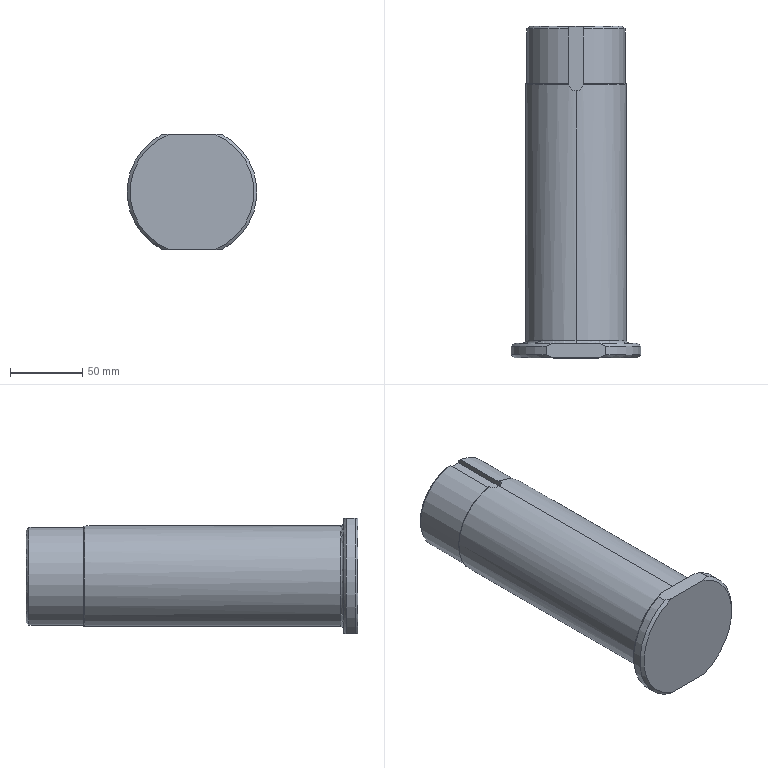Part | SolidWorks | features Fillet 3, ICE 2, Chamfer 1, Revolution 1 | 1 solid | 27 faces | box 90 x 230 x 80 mm | volume 896064 mm3 | plane 9 | cylinder 8 | cone 6 | torus 4 | commonest cylinder face diameters 10 x2 68 x2 70 x2 90 x2
STEP:
#1=CARTESIAN_POINT('',(0.,190.,-34.5));
#2=VERTEX_POINT('',#1);
#3=CARTESIAN_POINT('',(-5.,190.,34.136));
#4=VERTEX_POINT('',#3);
#5=CARTESIAN_POINT('',(0.,190.,0.));
#6=DIRECTION('',(0.,1.,0.));
#7=DIRECTION('',(0.,0.,-1.));
#8=AXIS2_PLACEMENT_3D('',#5,#6,#7);
#9=CIRCLE('',#8,34.5);
#10=EDGE_CURVE('',#2,#4,#9,.T.);
#11=ORIENTED_EDGE('',*,*,#10,.F.);
#12=CARTESIAN_POINT('',(0.,189.5,-35.));
#13=VERTEX_POINT('',#12);
#14=CARTESIAN_POINT('',(0.,189.5,-34.5));
#15=DIRECTION('',(-1.,0.,0.));
#16=DIRECTION('',(0.,0.,1.));
#17=AXIS2_PLACEMENT_3D('',#14,#15,#16);
#18=CIRCLE('',#17,0.5);
#19=EDGE_CURVE('',#2,#13,#18,.T.);
#20=ORIENTED_EDGE('',*,*,#19,.T.);
#21=CARTESIAN_POINT('',(-4.975,189.5,34.645));
#22=VERTEX_POINT('',#21);
#23=CARTESIAN_POINT('',(0.,189.5,0.));
#24=DIRECTION('',(0.,-1.,0.));
#25=DIRECTION('',(0.,0.,-1.));
#26=AXIS2_PLACEMENT_3D('',#23,#24,#25);
#27=CIRCLE('',#26,35.);
#28=EDGE_CURVE('',#22,#13,#27,.T.);
#29=ORIENTED_EDGE('',*,*,#28,.F.);
#30=CARTESIAN_POINT('',(-4.975,189.5,34.645));
#31=CARTESIAN_POINT('',(-4.988,189.632,34.643));
#32=CARTESIAN_POINT('',(-4.995,189.762,34.587));
#33=CARTESIAN_POINT('',(-5.001,189.946,34.399));
#34=CARTESIAN_POINT('',(-5.,190.,34.269));
#35=CARTESIAN_POINT('',(-5.,190.,34.136));
#36=B_SPLINE_CURVE_WITH_KNOTS('',3,(#30,#31,#32,#33,#34,#35),.UNSPECIFIED.,.F.,.F.,(4,2,4),(0.,0.0003936,0.0007872),.UNSPECIFIED.);
#37=EDGE_CURVE('',#22,#4,#36,.T.);
#38=ORIENTED_EDGE('',*,*,#37,.T.);
#39=EDGE_LOOP('',(#11,#20,#29,#38));
#40=FACE_OUTER_BOUND('',#39,.T.);
#41=CARTESIAN_POINT('',(0.,189.5,0.));
#42=DIRECTION('',(0.,-1.,0.));
#43=DIRECTION('',(0.,0.,-1.));
#44=AXIS2_PLACEMENT_3D('',#41,#42,#43);
#45=TOROIDAL_SURFACE('',#44,34.5,0.5);
#46=ADVANCED_FACE('',(#40),#45,.T.);
#47=CARTESIAN_POINT('',(0.,10.,37.));
#48=VERTEX_POINT('',#47);
#49=CARTESIAN_POINT('',(0.,10.,-37.));
#50=VERTEX_POINT('',#49);
#51=CARTESIAN_POINT('',(0.,10.,0.));
#52=DIRECTION('',(0.,-1.,0.));
#53=DIRECTION('',(0.,0.,-1.));
#54=AXIS2_PLACEMENT_3D('',#51,#52,#53);
#55=CIRCLE('',#54,37.);
#56=EDGE_CURVE('',#48,#50,#55,.T.);
#57=ORIENTED_EDGE('',*,*,#56,.F.);
#58=CARTESIAN_POINT('',(0.,12.,35.));
#59=VERTEX_POINT('',#58);
#60=CARTESIAN_POINT('',(0.,12.,37.));
#61=DIRECTION('',(1.,0.,0.));
#62=DIRECTION('',(0.,0.,-1.));
#63=AXIS2_PLACEMENT_3D('',#60,#61,#62);
#64=CIRCLE('',#63,2.);
#65=EDGE_CURVE('',#48,#59,#64,.T.);
#66=ORIENTED_EDGE('',*,*,#65,.T.);
#67=CARTESIAN_POINT('',(0.,12.,-35.));
#68=VERTEX_POINT('',#67);
#69=CARTESIAN_POINT('',(0.,12.,0.));
#70=DIRECTION('',(0.,1.,0.));
#71=DIRECTION('',(0.,0.,-1.));
#72=AXIS2_PLACEMENT_3D('',#69,#70,#71);
#73=CIRCLE('',#72,35.);
#74=EDGE_CURVE('',#68,#59,#73,.T.);
#75=ORIENTED_EDGE('',*,*,#74,.F.);
#76=CARTESIAN_POINT('',(0.,12.,-37.));
#77=DIRECTION('',(-1.,0.,0.));
#78=DIRECTION('',(0.,0.,1.));
#79=AXIS2_PLACEMENT_3D('',#76,#77,#78);
#80=CIRCLE('',#79,2.);
#81=EDGE_CURVE('',#50,#68,#80,.T.);
#82=ORIENTED_EDGE('',*,*,#81,.F.);
#83=EDGE_LOOP('',(#57,#66,#75,#82));
#84=FACE_OUTER_BOUND('',#83,.T.);
#85=CARTESIAN_POINT('',(0.,12.,0.));
#86=DIRECTION('',(0.,-1.,0.));
#87=DIRECTION('',(0.,0.,-1.));
#88=AXIS2_PLACEMENT_3D('',#85,#86,#87);
#89=TOROIDAL_SURFACE('',#88,37.,2.);
#90=ADVANCED_FACE('',(#84),#89,.F.);
#91=CARTESIAN_POINT('',(0.,230.,-32.));
#92=VERTEX_POINT('',#91);
#93=CARTESIAN_POINT('',(-5.,230.,31.607));
#94=VERTEX_POINT('',#93);
#95=CARTESIAN_POINT('',(0.,230.,0.));
#96=DIRECTION('',(0.,1.,0.));
#97=DIRECTION('',(0.,0.,-1.));
#98=AXIS2_PLACEMENT_3D('',#95,#96,#97);
#99=CIRCLE('',#98,32.);
#100=EDGE_CURVE('',#92,#94,#99,.T.);
#101=ORIENTED_EDGE('',*,*,#100,.F.);
#102=CARTESIAN_POINT('',(0.,228.,-34.));
#103=VERTEX_POINT('',#102);
#104=CARTESIAN_POINT('',(0.,228.,-34.));
#105=DIRECTION('',(0.,-0.7071,-0.7071));
#106=VECTOR('',#105,1000.);
#107=LINE('',#104,#106);
#108=EDGE_CURVE('',#92,#103,#107,.T.);
#109=ORIENTED_EDGE('',*,*,#108,.T.);
#110=CARTESIAN_POINT('',(-5.,228.,33.63));
#111=VERTEX_POINT('',#110);
#112=CARTESIAN_POINT('',(0.,228.,0.));
#113=DIRECTION('',(0.,-1.,0.));
#114=DIRECTION('',(0.,0.,-1.));
#115=AXIS2_PLACEMENT_3D('',#112,#113,#114);
#116=CIRCLE('',#115,34.);
#117=EDGE_CURVE('',#111,#103,#116,.T.);
#118=ORIENTED_EDGE('',*,*,#117,.F.);
#119=CARTESIAN_POINT('',(-5.,230.,31.607));
#120=CARTESIAN_POINT('',(-5.,229.334,32.282));
#121=CARTESIAN_POINT('',(-5.,228.667,32.956));
#122=CARTESIAN_POINT('',(-5.,228.,33.63));
#123=B_SPLINE_CURVE_WITH_KNOTS('',3,(#119,#120,#121,#122),.UNSPECIFIED.,.F.,.F.,(4,4),(0.006371,0.009216),.UNSPECIFIED.);
#124=EDGE_CURVE('',#94,#111,#123,.T.);
#125=ORIENTED_EDGE('',*,*,#124,.F.);
#126=EDGE_LOOP('',(#101,#109,#118,#125));
#127=FACE_OUTER_BOUND('',#126,.T.);
#128=CARTESIAN_POINT('',(0.,228.,0.));
#129=DIRECTION('',(0.,-1.,0.));
#130=DIRECTION('',(0.,0.,-1.));
#131=AXIS2_PLACEMENT_3D('',#128,#129,#130);
#132=CONICAL_SURFACE('',#131,34.,0.7854);
#133=ADVANCED_FACE('',(#127),#132,.T.);
#134=ORIENTED_EDGE('',*,*,#117,.T.);
#135=CARTESIAN_POINT('',(0.,190.,-34.));
#136=VERTEX_POINT('',#135);
#137=CARTESIAN_POINT('',(0.,0.,-34.));
#138=DIRECTION('',(0.,-1.,0.));
#139=VECTOR('',#138,1000.);
#140=LINE('',#137,#139);
#141=EDGE_CURVE('',#103,#136,#140,.T.);
#142=ORIENTED_EDGE('',*,*,#141,.T.);
#143=CARTESIAN_POINT('',(-5.,190.,33.63));
#144=VERTEX_POINT('',#143);
#145=CARTESIAN_POINT('',(0.,190.,0.));
#146=DIRECTION('',(0.,-1.,0.));
#147=DIRECTION('',(0.,0.,-1.));
#148=AXIS2_PLACEMENT_3D('',#145,#146,#147);
#149=CIRCLE('',#148,34.);
#150=EDGE_CURVE('',#144,#136,#149,.T.);
#151=ORIENTED_EDGE('',*,*,#150,.F.);
#152=CARTESIAN_POINT('',(-5.,0.,33.63));
#153=DIRECTION('',(0.,-1.,0.));
#154=VECTOR('',#153,1000.);
#155=LINE('',#152,#154);
#156=EDGE_CURVE('',#111,#144,#155,.T.);
#157=ORIENTED_EDGE('',*,*,#156,.F.);
#158=EDGE_LOOP('',(#134,#142,#151,#157));
#159=FACE_OUTER_BOUND('',#158,.T.);
#160=CARTESIAN_POINT('',(0.,0.,0.));
#161=DIRECTION('',(0.,-1.,0.));
#162=DIRECTION('',(0.,0.,-1.));
#163=AXIS2_PLACEMENT_3D('',#160,#161,#162);
#164=CYLINDRICAL_SURFACE('',#163,34.);
#165=ADVANCED_FACE('',(#159),#164,.T.);
#166=CARTESIAN_POINT('',(4.975,189.5,34.645));
#167=VERTEX_POINT('',#166);
#168=CARTESIAN_POINT('',(0.,185.,35.));
#169=VERTEX_POINT('',#168);
#170=CARTESIAN_POINT('',(4.975,189.5,34.645));
#171=CARTESIAN_POINT('',(4.944,189.192,34.649));
#172=CARTESIAN_POINT('',(4.885,188.892,34.658));
#173=CARTESIAN_POINT('',(4.714,188.306,34.681));
#174=CARTESIAN_POINT('',(4.601,188.019,34.697));
#175=CARTESIAN_POINT('',(4.324,187.47,34.732));
#176=CARTESIAN_POINT('',(4.162,187.212,34.752));
#177=CARTESIAN_POINT('',(3.792,186.727,34.794));
#178=CARTESIAN_POINT('',(3.582,186.498,34.817));
#179=CARTESIAN_POINT('',(3.128,186.088,34.861));
#180=CARTESIAN_POINT('',(2.885,185.905,34.882));
#181=CARTESIAN_POINT('',(2.365,185.584,34.921));
#182=CARTESIAN_POINT('',(2.086,185.446,34.939));
#183=CARTESIAN_POINT('',(1.516,185.226,34.968));
#184=CARTESIAN_POINT('',(1.223,185.142,34.98));
#185=CARTESIAN_POINT('',(0.6195,185.029,34.996));
#186=CARTESIAN_POINT('',(0.3096,185.,35.));
#187=CARTESIAN_POINT('',(0.,185.,35.));
#188=B_SPLINE_CURVE_WITH_KNOTS('',3,(#170,#171,#172,#173,#174,#175,#176,#177,#178,#179,#180,#181,#182,#183,#184,#185,#186,#187),.UNSPECIFIED.,.F.,.F.,(4,2,2,2,2,2,2,2,4),(0.,0.0009154,0.001831,0.002746,0.003662,0.004577,0.005492,0.006408,0.007323),.UNSPECIFIED.);
#189=EDGE_CURVE('',#167,#169,#188,.T.);
#190=ORIENTED_EDGE('',*,*,#189,.T.);
#191=CARTESIAN_POINT('',(0.,0.,35.));
#192=DIRECTION('',(0.,-1.,0.));
#193=VECTOR('',#192,1000.);
#194=LINE('',#191,#193);
#195=EDGE_CURVE('',#169,#59,#194,.T.);
#196=ORIENTED_EDGE('',*,*,#195,.T.);
#197=CARTESIAN_POINT('',(0.,12.,0.));
#198=DIRECTION('',(0.,1.,0.));
#199=DIRECTION('',(0.,0.,-1.));
#200=AXIS2_PLACEMENT_3D('',#197,#198,#199);
#201=CIRCLE('',#200,35.);
#202=EDGE_CURVE('',#59,#68,#201,.T.);
#203=ORIENTED_EDGE('',*,*,#202,.T.);
#204=CARTESIAN_POINT('',(0.,0.,-35.));
#205=DIRECTION('',(0.,-1.,0.));
#206=VECTOR('',#205,1000.);
#207=LINE('',#204,#206);
#208=EDGE_CURVE('',#13,#68,#207,.T.);
#209=ORIENTED_EDGE('',*,*,#208,.F.);
#210=CARTESIAN_POINT('',(0.,189.5,0.));
#211=DIRECTION('',(0.,-1.,0.));
#212=DIRECTION('',(0.,0.,-1.));
#213=AXIS2_PLACEMENT_3D('',#210,#211,#212);
#214=CIRCLE('',#213,35.);
#215=EDGE_CURVE('',#13,#167,#214,.T.);
#216=ORIENTED_EDGE('',*,*,#215,.T.);
#217=EDGE_LOOP('',(#190,#196,#203,#209,#216));
#218=FACE_OUTER_BOUND('',#217,.T.);
#219=CARTESIAN_POINT('',(0.,0.,0.));
#220=DIRECTION('',(0.,-1.,0.));
#221=DIRECTION('',(0.,0.,-1.));
#222=AXIS2_PLACEMENT_3D('',#219,#220,#221);
#223=CYLINDRICAL_SURFACE('',#222,35.);
#224=ADVANCED_FACE('',(#218),#223,.T.);
#225=CARTESIAN_POINT('',(20.616,8.,-40.));
#226=VERTEX_POINT('',#225);
#227=CARTESIAN_POINT('',(20.616,2.,-40.));
#228=VERTEX_POINT('',#227);
#229=CARTESIAN_POINT('',(20.616,0.,-40.));
#230=DIRECTION('',(0.,-1.,0.));
#231=VECTOR('',#230,1000.);
#232=LINE('',#229,#231);
#233=EDGE_CURVE('',#226,#228,#232,.T.);
#234=ORIENTED_EDGE('',*,*,#233,.F.);
#235=CARTESIAN_POINT('',(20.616,8.,40.));
#236=VERTEX_POINT('',#235);
#237=CARTESIAN_POINT('',(0.,8.,0.));
#238=DIRECTION('',(0.,-1.,0.));
#239=DIRECTION('',(0.,0.,-1.));
#240=AXIS2_PLACEMENT_3D('',#237,#238,#239);
#241=CIRCLE('',#240,45.);
#242=EDGE_CURVE('',#226,#236,#241,.T.);
#243=ORIENTED_EDGE('',*,*,#242,.T.);
#244=CARTESIAN_POINT('',(20.616,2.,40.));
#245=VERTEX_POINT('',#244);
#246=CARTESIAN_POINT('',(20.616,0.,40.));
#247=DIRECTION('',(0.,1.,0.));
#248=VECTOR('',#247,1000.);
#249=LINE('',#246,#248);
#250=EDGE_CURVE('',#245,#236,#249,.T.);
#251=ORIENTED_EDGE('',*,*,#250,.F.);
#252=CARTESIAN_POINT('',(0.,2.,0.));
#253=DIRECTION('',(0.,1.,0.));
#254=DIRECTION('',(0.,0.,-1.));
#255=AXIS2_PLACEMENT_3D('',#252,#253,#254);
#256=CIRCLE('',#255,45.);
#257=EDGE_CURVE('',#245,#228,#256,.T.);
#258=ORIENTED_EDGE('',*,*,#257,.T.);
#259=EDGE_LOOP('',(#234,#243,#251,#258));
#260=FACE_OUTER_BOUND('',#259,.T.);
#261=CARTESIAN_POINT('',(0.,0.,0.));
#262=DIRECTION('',(0.,-1.,0.));
#263=DIRECTION('',(0.,0.,-1.));
#264=AXIS2_PLACEMENT_3D('',#261,#262,#263);
#265=CYLINDRICAL_SURFACE('',#264,45.);
#266=ADVANCED_FACE('',(#260),#265,.T.);
#267=CARTESIAN_POINT('',(-20.616,8.,40.));
#268=VERTEX_POINT('',#267);
#269=CARTESIAN_POINT('',(-20.616,2.,40.));
#270=VERTEX_POINT('',#269);
#271=CARTESIAN_POINT('',(-20.616,0.,40.));
#272=DIRECTION('',(0.,-1.,0.));
#273=VECTOR('',#272,1000.);
#274=LINE('',#271,#273);
#275=EDGE_CURVE('',#268,#270,#274,.T.);
#276=ORIENTED_EDGE('',*,*,#275,.F.);
#277=CARTESIAN_POINT('',(-20.616,8.,-40.));
#278=VERTEX_POINT('',#277);
#279=CARTESIAN_POINT('',(0.,8.,0.));
#280=DIRECTION('',(0.,-1.,0.));
#281=DIRECTION('',(0.,0.,-1.));
#282=AXIS2_PLACEMENT_3D('',#279,#280,#281);
#283=CIRCLE('',#282,45.);
#284=EDGE_CURVE('',#268,#278,#283,.T.);
#285=ORIENTED_EDGE('',*,*,#284,.T.);
#286=CARTESIAN_POINT('',(-20.616,2.,-40.));
#287=VERTEX_POINT('',#286);
#288=CARTESIAN_POINT('',(-20.616,0.,-40.));
#289=DIRECTION('',(0.,1.,0.));
#290=VECTOR('',#289,1000.);
#291=LINE('',#288,#290);
#292=EDGE_CURVE('',#287,#278,#291,.T.);
#293=ORIENTED_EDGE('',*,*,#292,.F.);
#294=CARTESIAN_POINT('',(0.,2.,0.));
#295=DIRECTION('',(0.,1.,0.));
#296=DIRECTION('',(0.,0.,-1.));
#297=AXIS2_PLACEMENT_3D('',#294,#295,#296);
#298=CIRCLE('',#297,45.);
#299=EDGE_CURVE('',#287,#270,#298,.T.);
#300=ORIENTED_EDGE('',*,*,#299,.T.);
#301=EDGE_LOOP('',(#276,#285,#293,#300));
#302=FACE_OUTER_BOUND('',#301,.T.);
#303=CARTESIAN_POINT('',(0.,0.,0.));
#304=DIRECTION('',(0.,-1.,0.));
#305=DIRECTION('',(0.,0.,-1.));
#306=AXIS2_PLACEMENT_3D('',#303,#304,#305);
#307=CYLINDRICAL_SURFACE('',#306,45.);
#308=ADVANCED_FACE('',(#302),#307,.T.);
#309=CARTESIAN_POINT('',(15.78,0.,-40.));
#310=VERTEX_POINT('',#309);
#311=CARTESIAN_POINT('',(-15.78,0.,-40.));
#312=VERTEX_POINT('',#311);
#313=CARTESIAN_POINT('',(0.,0.,-40.));
#314=DIRECTION('',(-1.,0.,0.));
#315=VECTOR('',#314,1000.);
#316=LINE('',#313,#315);
#317=EDGE_CURVE('',#310,#312,#316,.T.);
#318=ORIENTED_EDGE('',*,*,#317,.F.);
#319=CARTESIAN_POINT('',(15.78,0.,40.));
#320=VERTEX_POINT('',#319);
#321=CARTESIAN_POINT('',(0.,0.,0.));
#322=DIRECTION('',(0.,-1.,0.));
#323=DIRECTION('',(0.,0.,-1.));
#324=AXIS2_PLACEMENT_3D('',#321,#322,#323);
#325=CIRCLE('',#324,43.);
#326=EDGE_CURVE('',#310,#320,#325,.T.);
#327=ORIENTED_EDGE('',*,*,#326,.T.);
#328=CARTESIAN_POINT('',(-15.78,0.,40.));
#329=VERTEX_POINT('',#328);
#330=CARTESIAN_POINT('',(0.,0.,40.));
#331=DIRECTION('',(1.,0.,0.));
#332=VECTOR('',#331,1000.);
#333=LINE('',#330,#332);
#334=EDGE_CURVE('',#329,#320,#333,.T.);
#335=ORIENTED_EDGE('',*,*,#334,.F.);
#336=CARTESIAN_POINT('',(0.,0.,0.));
#337=DIRECTION('',(0.,-1.,0.));
#338=DIRECTION('',(0.,0.,-1.));
#339=AXIS2_PLACEMENT_3D('',#336,#337,#338);
#340=CIRCLE('',#339,43.);
#341=EDGE_CURVE('',#329,#312,#340,.T.);
#342=ORIENTED_EDGE('',*,*,#341,.T.);
#343=EDGE_LOOP('',(#318,#327,#335,#342));
#344=FACE_OUTER_BOUND('',#343,.T.);
#345=CARTESIAN_POINT('',(0.,0.,0.));
#346=DIRECTION('',(0.,-1.,0.));
#347=DIRECTION('',(0.,0.,-1.));
#348=AXIS2_PLACEMENT_3D('',#345,#346,#347);
#349=PLANE('',#348);
#350=ADVANCED_FACE('',(#344),#349,.T.);
#351=CARTESIAN_POINT('',(0.,10.,0.));
#352=DIRECTION('',(0.,-1.,0.));
#353=DIRECTION('',(0.,0.,-1.));
#354=AXIS2_PLACEMENT_3D('',#351,#352,#353);
#355=CIRCLE('',#354,37.);
#356=EDGE_CURVE('',#50,#48,#355,.T.);
#357=ORIENTED_EDGE('',*,*,#356,.T.);
#358=ORIENTED_EDGE('',*,*,#56,.T.);
#359=EDGE_LOOP('',(#357,#358));
#360=FACE_BOUND('',#359,.T.);
#361=CARTESIAN_POINT('',(15.78,10.,-40.));
#362=VERTEX_POINT('',#361);
#363=CARTESIAN_POINT('',(-15.78,10.,-40.));
#364=VERTEX_POINT('',#363);
#365=CARTESIAN_POINT('',(0.,10.,-40.));
#366=DIRECTION('',(-1.,0.,0.));
#367=VECTOR('',#366,1000.);
#368=LINE('',#365,#367);
#369=EDGE_CURVE('',#362,#364,#368,.T.);
#370=ORIENTED_EDGE('',*,*,#369,.T.);
#371=CARTESIAN_POINT('',(-15.78,10.,40.));
#372=VERTEX_POINT('',#371);
#373=CARTESIAN_POINT('',(0.,10.,0.));
#374=DIRECTION('',(0.,1.,0.));
#375=DIRECTION('',(0.,0.,-1.));
#376=AXIS2_PLACEMENT_3D('',#373,#374,#375);
#377=CIRCLE('',#376,43.);
#378=EDGE_CURVE('',#364,#372,#377,.T.);
#379=ORIENTED_EDGE('',*,*,#378,.T.);
#380=CARTESIAN_POINT('',(15.78,10.,40.));
#381=VERTEX_POINT('',#380);
#382=CARTESIAN_POINT('',(0.,10.,40.));
#383=DIRECTION('',(1.,0.,0.));
#384=VECTOR('',#383,1000.);
#385=LINE('',#382,#384);
#386=EDGE_CURVE('',#372,#381,#385,.T.);
#387=ORIENTED_EDGE('',*,*,#386,.T.);
#388=CARTESIAN_POINT('',(0.,10.,0.));
#389=DIRECTION('',(0.,1.,0.));
#390=DIRECTION('',(0.,0.,-1.));
#391=AXIS2_PLACEMENT_3D('',#388,#389,#390);
#392=CIRCLE('',#391,43.);
#393=EDGE_CURVE('',#381,#362,#392,.T.);
#394=ORIENTED_EDGE('',*,*,#393,.T.);
#395=EDGE_LOOP('',(#370,#379,#387,#394));
#396=FACE_OUTER_BOUND('',#395,.T.);
#397=CARTESIAN_POINT('',(0.,10.,0.));
#398=DIRECTION('',(0.,-1.,0.));
#399=DIRECTION('',(0.,0.,-1.));
#400=AXIS2_PLACEMENT_3D('',#397,#398,#399);
#401=PLANE('',#400);
#402=ADVANCED_FACE('',(#360,#396),#401,.F.);
#403=ORIENTED_EDGE('',*,*,#150,.T.);
#404=CARTESIAN_POINT('',(5.,190.,33.63));
#405=VERTEX_POINT('',#404);
#406=CARTESIAN_POINT('',(0.,190.,0.));
#407=DIRECTION('',(0.,-1.,0.));
#408=DIRECTION('',(0.,0.,-1.));
#409=AXIS2_PLACEMENT_3D('',#406,#407,#408);
#410=CIRCLE('',#409,34.);
#411=EDGE_CURVE('',#136,#405,#410,.T.);
#412=ORIENTED_EDGE('',*,*,#411,.T.);
#413=CARTESIAN_POINT('',(5.,190.,34.136));
#414=VERTEX_POINT('',#413);
#415=CARTESIAN_POINT('',(5.,190.,0.));
#416=DIRECTION('',(0.,0.,1.));
#417=VECTOR('',#416,1000.);
#418=LINE('',#415,#417);
#419=EDGE_CURVE('',#405,#414,#418,.T.);
#420=ORIENTED_EDGE('',*,*,#419,.T.);
#421=CARTESIAN_POINT('',(0.,190.,0.));
#422=DIRECTION('',(0.,1.,0.));
#423=DIRECTION('',(0.,0.,-1.));
#424=AXIS2_PLACEMENT_3D('',#421,#422,#423);
#425=CIRCLE('',#424,34.5);
#426=EDGE_CURVE('',#414,#2,#425,.T.);
#427=ORIENTED_EDGE('',*,*,#426,.T.);
#428=ORIENTED_EDGE('',*,*,#10,.T.);
#429=CARTESIAN_POINT('',(-5.,190.,0.));
#430=DIRECTION('',(0.,0.,-1.));
#431=VECTOR('',#430,1000.);
#432=LINE('',#429,#431);
#433=EDGE_CURVE('',#4,#144,#432,.T.);
#434=ORIENTED_EDGE('',*,*,#433,.T.);
#435=EDGE_LOOP('',(#403,#412,#420,#427,#428,#434));
#436=FACE_OUTER_BOUND('',#435,.T.);
#437=CARTESIAN_POINT('',(0.,190.,0.));
#438=DIRECTION('',(0.,-1.,0.));
#439=DIRECTION('',(0.,0.,-1.));
#440=AXIS2_PLACEMENT_3D('',#437,#438,#439);
#441=PLANE('',#440);
#442=ADVANCED_FACE('',(#436),#441,.F.);
#443=CARTESIAN_POINT('',(5.,230.,30.));
#444=VERTEX_POINT('',#443);
#445=CARTESIAN_POINT('',(-5.,230.,30.));
#446=VERTEX_POINT('',#445);
#447=CARTESIAN_POINT('',(-5.,230.,30.));
#448=DIRECTION('',(-1.,0.,0.));
#449=VECTOR('',#448,1000.);
#450=LINE('',#447,#449);
#451=EDGE_CURVE('',#444,#446,#450,.T.);
#452=ORIENTED_EDGE('',*,*,#451,.F.);
#453=CARTESIAN_POINT('',(5.,230.,31.607));
#454=VERTEX_POINT('',#453);
#455=CARTESIAN_POINT('',(5.,230.,77.437));
#456=DIRECTION('',(0.,0.,-1.));
#457=VECTOR('',#456,1000.);
#458=LINE('',#455,#457);
#459=EDGE_CURVE('',#454,#444,#458,.T.);
#460=ORIENTED_EDGE('',*,*,#459,.F.);
#461=CARTESIAN_POINT('',(0.,230.,0.));
#462=DIRECTION('',(0.,1.,0.));
#463=DIRECTION('',(0.,0.,-1.));
#464=AXIS2_PLACEMENT_3D('',#461,#462,#463);
#465=CIRCLE('',#464,32.);
#466=EDGE_CURVE('',#454,#92,#465,.T.);
#467=ORIENTED_EDGE('',*,*,#466,.T.);
#468=ORIENTED_EDGE('',*,*,#100,.T.);
#469=CARTESIAN_POINT('',(-5.,230.,77.437));
#470=DIRECTION('',(0.,0.,1.));
#471=VECTOR('',#470,1000.);
#472=LINE('',#469,#471);
#473=EDGE_CURVE('',#446,#94,#472,.T.);
#474=ORIENTED_EDGE('',*,*,#473,.F.);
#475=EDGE_LOOP('',(#452,#460,#467,#468,#474));
#476=FACE_OUTER_BOUND('',#475,.T.);
#477=CARTESIAN_POINT('',(0.,230.,0.));
#478=DIRECTION('',(0.,-1.,0.));
#479=DIRECTION('',(0.,0.,-1.));
#480=AXIS2_PLACEMENT_3D('',#477,#478,#479);
#481=PLANE('',#480);
#482=ADVANCED_FACE('',(#476),#481,.F.);
#483=ORIENTED_EDGE('',*,*,#141,.F.);
#484=CARTESIAN_POINT('',(5.,228.,33.63));
#485=VERTEX_POINT('',#484);
#486=CARTESIAN_POINT('',(0.,228.,0.));
#487=DIRECTION('',(0.,-1.,0.));
#488=DIRECTION('',(0.,0.,-1.));
#489=AXIS2_PLACEMENT_3D('',#486,#487,#488);
#490=CIRCLE('',#489,34.);
#491=EDGE_CURVE('',#103,#485,#490,.T.);
#492=ORIENTED_EDGE('',*,*,#491,.T.);
#493=CARTESIAN_POINT('',(5.,0.,33.63));
#494=DIRECTION('',(0.,1.,0.));
#495=VECTOR('',#494,1000.);
#496=LINE('',#493,#495);
#497=EDGE_CURVE('',#405,#485,#496,.T.);
#498=ORIENTED_EDGE('',*,*,#497,.F.);
#499=ORIENTED_EDGE('',*,*,#411,.F.);
#500=EDGE_LOOP('',(#483,#492,#498,#499));
#501=FACE_OUTER_BOUND('',#500,.T.);
#502=CARTESIAN_POINT('',(0.,0.,0.));
#503=DIRECTION('',(0.,-1.,0.));
#504=DIRECTION('',(0.,0.,-1.));
#505=AXIS2_PLACEMENT_3D('',#502,#503,#504);
#506=CYLINDRICAL_SURFACE('',#505,34.);
#507=ADVANCED_FACE('',(#501),#506,.T.);
#508=ORIENTED_EDGE('',*,*,#195,.F.);
#509=CARTESIAN_POINT('',(0.,185.,35.));
#510=CARTESIAN_POINT('',(-0.3096,185.,35.));
#511=CARTESIAN_POINT('',(-0.6142,185.028,34.996));
#512=CARTESIAN_POINT('',(-1.214,185.14,34.98));
#513=CARTESIAN_POINT('',(-1.512,185.224,34.969));
#514=CARTESIAN_POINT('',(-2.086,185.445,34.939));
#515=CARTESIAN_POINT('',(-2.359,185.581,34.921));
#516=CARTESIAN_POINT('',(-2.878,185.9,34.882));
#517=CARTESIAN_POINT('',(-3.127,186.086,34.861));
#518=CARTESIAN_POINT('',(-3.581,186.497,34.817));
#519=CARTESIAN_POINT('',(-3.787,186.721,34.795));
#520=CARTESIAN_POINT('',(-4.158,187.206,34.753));
#521=CARTESIAN_POINT('',(-4.323,187.47,34.732));
#522=CARTESIAN_POINT('',(-4.599,188.015,34.697));
#523=CARTESIAN_POINT('',(-4.711,188.298,34.682));
#524=CARTESIAN_POINT('',(-4.884,188.887,34.658));
#525=CARTESIAN_POINT('',(-4.944,189.192,34.649));
#526=CARTESIAN_POINT('',(-4.975,189.5,34.645));
#527=B_SPLINE_CURVE_WITH_KNOTS('',3,(#509,#510,#511,#512,#513,#514,#515,#516,#517,#518,#519,#520,#521,#522,#523,#524,#525,#526),.UNSPECIFIED.,.F.,.F.,(4,2,2,2,2,2,2,2,4),(0.,0.0009154,0.001831,0.002746,0.003662,0.004577,0.005492,0.006408,0.007323),.UNSPECIFIED.);
#528=EDGE_CURVE('',#169,#22,#527,.T.);
#529=ORIENTED_EDGE('',*,*,#528,.T.);
#530=ORIENTED_EDGE('',*,*,#28,.T.);
#531=ORIENTED_EDGE('',*,*,#208,.T.);
#532=ORIENTED_EDGE('',*,*,#74,.T.);
#533=EDGE_LOOP('',(#508,#529,#530,#531,#532));
#534=FACE_OUTER_BOUND('',#533,.T.);
#535=CARTESIAN_POINT('',(0.,0.,0.));
#536=DIRECTION('',(0.,-1.,0.));
#537=DIRECTION('',(0.,0.,-1.));
#538=AXIS2_PLACEMENT_3D('',#535,#536,#537);
#539=CYLINDRICAL_SURFACE('',#538,35.);
#540=ADVANCED_FACE('',(#534),#539,.T.);
#541=ORIENTED_EDGE('',*,*,#292,.T.);
#542=CARTESIAN_POINT('',(-20.616,8.,-40.));
#543=CARTESIAN_POINT('',(-19.029,8.727,-40.));
#544=CARTESIAN_POINT('',(-17.419,9.399,-40.));
#545=CARTESIAN_POINT('',(-15.78,10.,-40.));
#546=B_SPLINE_CURVE_WITH_KNOTS('',3,(#542,#543,#544,#545),.UNSPECIFIED.,.F.,.F.,(4,4),(0.,0.005233),.UNSPECIFIED.);
#547=EDGE_CURVE('',#278,#364,#546,.T.);
#548=ORIENTED_EDGE('',*,*,#547,.T.);
#549=ORIENTED_EDGE('',*,*,#369,.F.);
#550=CARTESIAN_POINT('',(15.78,10.,-40.));
#551=CARTESIAN_POINT('',(17.419,9.399,-40.));
#552=CARTESIAN_POINT('',(19.029,8.727,-40.));
#553=CARTESIAN_POINT('',(20.616,8.,-40.));
#554=B_SPLINE_CURVE_WITH_KNOTS('',3,(#550,#551,#552,#553),.UNSPECIFIED.,.F.,.F.,(4,4),(0.,0.005233),.UNSPECIFIED.);
#555=EDGE_CURVE('',#362,#226,#554,.T.);
#556=ORIENTED_EDGE('',*,*,#555,.T.);
#557=ORIENTED_EDGE('',*,*,#233,.T.);
#558=CARTESIAN_POINT('',(20.616,2.,-40.));
#559=CARTESIAN_POINT('',(19.029,1.273,-40.));
#560=CARTESIAN_POINT('',(17.419,0.6014,-40.));
#561=CARTESIAN_POINT('',(15.78,0.,-40.));
#562=B_SPLINE_CURVE_WITH_KNOTS('',3,(#558,#559,#560,#561),.UNSPECIFIED.,.F.,.F.,(4,4),(0.,0.005233),.UNSPECIFIED.);
#563=EDGE_CURVE('',#228,#310,#562,.T.);
#564=ORIENTED_EDGE('',*,*,#563,.T.);
#565=ORIENTED_EDGE('',*,*,#317,.T.);
#566=CARTESIAN_POINT('',(-15.78,0.,-40.));
#567=CARTESIAN_POINT('',(-17.419,0.6014,-40.));
#568=CARTESIAN_POINT('',(-19.029,1.273,-40.));
#569=CARTESIAN_POINT('',(-20.616,2.,-40.));
#570=B_SPLINE_CURVE_WITH_KNOTS('',3,(#566,#567,#568,#569),.UNSPECIFIED.,.F.,.F.,(4,4),(0.,0.005233),.UNSPECIFIED.);
#571=EDGE_CURVE('',#312,#287,#570,.T.);
#572=ORIENTED_EDGE('',*,*,#571,.T.);
#573=EDGE_LOOP('',(#541,#548,#549,#556,#557,#564,#565,#572));
#574=FACE_OUTER_BOUND('',#573,.T.);
#575=CARTESIAN_POINT('',(-75.192,230.,-40.));
#576=DIRECTION('',(0.,0.,1.));
#577=DIRECTION('',(1.,0.,0.));
#578=AXIS2_PLACEMENT_3D('',#575,#576,#577);
#579=PLANE('',#578);
#580=ADVANCED_FACE('',(#574),#579,.F.);
#581=ORIENTED_EDGE('',*,*,#386,.F.);
#582=CARTESIAN_POINT('',(-15.78,10.,40.));
#583=CARTESIAN_POINT('',(-17.419,9.399,40.));
#584=CARTESIAN_POINT('',(-19.029,8.727,40.));
#585=CARTESIAN_POINT('',(-20.616,8.,40.));
#586=B_SPLINE_CURVE_WITH_KNOTS('',3,(#582,#583,#584,#585),.UNSPECIFIED.,.F.,.F.,(4,4),(0.,0.005233),.UNSPECIFIED.);
#587=EDGE_CURVE('',#372,#268,#586,.T.);
#588=ORIENTED_EDGE('',*,*,#587,.T.);
#589=ORIENTED_EDGE('',*,*,#275,.T.);
#590=CARTESIAN_POINT('',(-20.616,2.,40.));
#591=CARTESIAN_POINT('',(-19.029,1.273,40.));
#592=CARTESIAN_POINT('',(-17.419,0.6014,40.));
#593=CARTESIAN_POINT('',(-15.78,0.,40.));
#594=B_SPLINE_CURVE_WITH_KNOTS('',3,(#590,#591,#592,#593),.UNSPECIFIED.,.F.,.F.,(4,4),(0.,0.005233),.UNSPECIFIED.);
#595=EDGE_CURVE('',#270,#329,#594,.T.);
#596=ORIENTED_EDGE('',*,*,#595,.T.);
#597=ORIENTED_EDGE('',*,*,#334,.T.);
#598=CARTESIAN_POINT('',(15.78,0.,40.));
#599=CARTESIAN_POINT('',(17.419,0.6014,40.));
#600=CARTESIAN_POINT('',(19.029,1.273,40.));
#601=CARTESIAN_POINT('',(20.616,2.,40.));
#602=B_SPLINE_CURVE_WITH_KNOTS('',3,(#598,#599,#600,#601),.UNSPECIFIED.,.F.,.F.,(4,4),(0.,0.005233),.UNSPECIFIED.);
#603=EDGE_CURVE('',#320,#245,#602,.T.);
#604=ORIENTED_EDGE('',*,*,#603,.T.);
#605=ORIENTED_EDGE('',*,*,#250,.T.);
#606=CARTESIAN_POINT('',(20.616,8.,40.));
#607=CARTESIAN_POINT('',(19.029,8.727,40.));
#608=CARTESIAN_POINT('',(17.419,9.399,40.));
#609=CARTESIAN_POINT('',(15.78,10.,40.));
#610=B_SPLINE_CURVE_WITH_KNOTS('',3,(#606,#607,#608,#609),.UNSPECIFIED.,.F.,.F.,(4,4),(0.,0.005233),.UNSPECIFIED.);
#611=EDGE_CURVE('',#236,#381,#610,.T.);
#612=ORIENTED_EDGE('',*,*,#611,.T.);
#613=EDGE_LOOP('',(#581,#588,#589,#596,#597,#604,#605,#612));
#614=FACE_OUTER_BOUND('',#613,.T.);
#615=CARTESIAN_POINT('',(-79.562,230.,40.));
#616=DIRECTION('',(0.,0.,-1.));
#617=DIRECTION('',(-1.,0.,0.));
#618=AXIS2_PLACEMENT_3D('',#615,#616,#617);
#619=PLANE('',#618);
#620=ADVANCED_FACE('',(#614),#619,.F.);
#621=ORIENTED_EDGE('',*,*,#108,.F.);
#622=ORIENTED_EDGE('',*,*,#466,.F.);
#623=CARTESIAN_POINT('',(5.,228.,33.63));
#624=CARTESIAN_POINT('',(5.,228.667,32.956));
#625=CARTESIAN_POINT('',(5.,229.334,32.282));
#626=CARTESIAN_POINT('',(5.,230.,31.607));
#627=B_SPLINE_CURVE_WITH_KNOTS('',3,(#623,#624,#625,#626),.UNSPECIFIED.,.F.,.F.,(4,4),(0.006356,0.009201),.UNSPECIFIED.);
#628=EDGE_CURVE('',#485,#454,#627,.T.);
#629=ORIENTED_EDGE('',*,*,#628,.F.);
#630=ORIENTED_EDGE('',*,*,#491,.F.);
#631=EDGE_LOOP('',(#621,#622,#629,#630));
#632=FACE_OUTER_BOUND('',#631,.T.);
#633=CARTESIAN_POINT('',(0.,228.,0.));
#634=DIRECTION('',(0.,-1.,0.));
#635=DIRECTION('',(0.,0.,-1.));
#636=AXIS2_PLACEMENT_3D('',#633,#634,#635);
#637=CONICAL_SURFACE('',#636,34.,0.7854);
#638=ADVANCED_FACE('',(#632),#637,.T.);
#639=ORIENTED_EDGE('',*,*,#587,.F.);
#640=ORIENTED_EDGE('',*,*,#378,.F.);
#641=ORIENTED_EDGE('',*,*,#547,.F.);
#642=ORIENTED_EDGE('',*,*,#284,.F.);
#643=EDGE_LOOP('',(#639,#640,#641,#642));
#644=FACE_OUTER_BOUND('',#643,.T.);
#645=CARTESIAN_POINT('',(0.,8.,0.));
#646=DIRECTION('',(0.,-1.,0.));
#647=DIRECTION('',(0.,0.,-1.));
#648=AXIS2_PLACEMENT_3D('',#645,#646,#647);
#649=CONICAL_SURFACE('',#648,45.,0.7854);
#650=ADVANCED_FACE('',(#644),#649,.T.);
#651=ORIENTED_EDGE('',*,*,#555,.F.);
#652=ORIENTED_EDGE('',*,*,#393,.F.);
#653=ORIENTED_EDGE('',*,*,#611,.F.);
#654=ORIENTED_EDGE('',*,*,#242,.F.);
#655=EDGE_LOOP('',(#651,#652,#653,#654));
#656=FACE_OUTER_BOUND('',#655,.T.);
#657=CARTESIAN_POINT('',(0.,8.,0.));
#658=DIRECTION('',(0.,-1.,0.));
#659=DIRECTION('',(0.,0.,-1.));
#660=AXIS2_PLACEMENT_3D('',#657,#658,#659);
#661=CONICAL_SURFACE('',#660,45.,0.7854);
#662=ADVANCED_FACE('',(#656),#661,.T.);
#663=ORIENTED_EDGE('',*,*,#563,.F.);
#664=ORIENTED_EDGE('',*,*,#257,.F.);
#665=ORIENTED_EDGE('',*,*,#603,.F.);
#666=ORIENTED_EDGE('',*,*,#326,.F.);
#667=EDGE_LOOP('',(#663,#664,#665,#666));
#668=FACE_OUTER_BOUND('',#667,.T.);
#669=CARTESIAN_POINT('',(0.,0.,0.));
#670=DIRECTION('',(0.,1.,0.));
#671=DIRECTION('',(0.,0.,1.));
#672=AXIS2_PLACEMENT_3D('',#669,#670,#671);
#673=CONICAL_SURFACE('',#672,43.,0.7854);
#674=ADVANCED_FACE('',(#668),#673,.T.);
#675=ORIENTED_EDGE('',*,*,#595,.F.);
#676=ORIENTED_EDGE('',*,*,#299,.F.);
#677=ORIENTED_EDGE('',*,*,#571,.F.);
#678=ORIENTED_EDGE('',*,*,#341,.F.);
#679=EDGE_LOOP('',(#675,#676,#677,#678));
#680=FACE_OUTER_BOUND('',#679,.T.);
#681=CARTESIAN_POINT('',(0.,0.,0.));
#682=DIRECTION('',(0.,1.,0.));
#683=DIRECTION('',(0.,0.,1.));
#684=AXIS2_PLACEMENT_3D('',#681,#682,#683);
#685=CONICAL_SURFACE('',#684,43.,0.7854);
#686=ADVANCED_FACE('',(#680),#685,.T.);
#687=ORIENTED_EDGE('',*,*,#65,.F.);
#688=ORIENTED_EDGE('',*,*,#356,.F.);
#689=ORIENTED_EDGE('',*,*,#81,.T.);
#690=ORIENTED_EDGE('',*,*,#202,.F.);
#691=EDGE_LOOP('',(#687,#688,#689,#690));
#692=FACE_OUTER_BOUND('',#691,.T.);
#693=CARTESIAN_POINT('',(0.,12.,0.));
#694=DIRECTION('',(0.,-1.,0.));
#695=DIRECTION('',(0.,0.,-1.));
#696=AXIS2_PLACEMENT_3D('',#693,#694,#695);
#697=TOROIDAL_SURFACE('',#696,37.,2.);
#698=ADVANCED_FACE('',(#692),#697,.F.);
#699=ORIENTED_EDGE('',*,*,#19,.F.);
#700=ORIENTED_EDGE('',*,*,#426,.F.);
#701=CARTESIAN_POINT('',(5.,190.,34.136));
#702=CARTESIAN_POINT('',(5.,190.,34.269));
#703=CARTESIAN_POINT('',(5.001,189.946,34.399));
#704=CARTESIAN_POINT('',(4.995,189.762,34.587));
#705=CARTESIAN_POINT('',(4.988,189.632,34.643));
#706=CARTESIAN_POINT('',(4.975,189.5,34.645));
#707=B_SPLINE_CURVE_WITH_KNOTS('',3,(#701,#702,#703,#704,#705,#706),.UNSPECIFIED.,.F.,.F.,(4,2,4),(0.,0.0003936,0.0007872),.UNSPECIFIED.);
#708=EDGE_CURVE('',#414,#167,#707,.T.);
#709=ORIENTED_EDGE('',*,*,#708,.T.);
#710=ORIENTED_EDGE('',*,*,#215,.F.);
#711=EDGE_LOOP('',(#699,#700,#709,#710));
#712=FACE_OUTER_BOUND('',#711,.T.);
#713=CARTESIAN_POINT('',(0.,189.5,0.));
#714=DIRECTION('',(0.,-1.,0.));
#715=DIRECTION('',(0.,0.,-1.));
#716=AXIS2_PLACEMENT_3D('',#713,#714,#715);
#717=TOROIDAL_SURFACE('',#716,34.5,0.5);
#718=ADVANCED_FACE('',(#712),#717,.T.);
#719=CARTESIAN_POINT('',(5.,190.,30.));
#720=VERTEX_POINT('',#719);
#721=CARTESIAN_POINT('',(5.,185.,30.));
#722=DIRECTION('',(0.,1.,0.));
#723=VECTOR('',#722,1000.);
#724=LINE('',#721,#723);
#725=EDGE_CURVE('',#720,#444,#724,.T.);
#726=ORIENTED_EDGE('',*,*,#725,.F.);
#727=CARTESIAN_POINT('',(5.,190.,34.641));
#728=DIRECTION('',(0.,0.,1.));
#729=VECTOR('',#728,1000.);
#730=LINE('',#727,#729);
#731=EDGE_CURVE('',#720,#405,#730,.T.);
#732=ORIENTED_EDGE('',*,*,#731,.T.);
#733=ORIENTED_EDGE('',*,*,#497,.T.);
#734=ORIENTED_EDGE('',*,*,#628,.T.);
#735=ORIENTED_EDGE('',*,*,#459,.T.);
#736=EDGE_LOOP('',(#726,#732,#733,#734,#735));
#737=FACE_OUTER_BOUND('',#736,.T.);
#738=CARTESIAN_POINT('',(5.,185.,77.437));
#739=DIRECTION('',(1.,0.,0.));
#740=DIRECTION('',(0.,0.,-1.));
#741=AXIS2_PLACEMENT_3D('',#738,#739,#740);
#742=PLANE('',#741);
#743=ADVANCED_FACE('',(#737),#742,.F.);
#744=ORIENTED_EDGE('',*,*,#156,.T.);
#745=CARTESIAN_POINT('',(-5.,190.,30.));
#746=VERTEX_POINT('',#745);
#747=CARTESIAN_POINT('',(-5.,190.,30.));
#748=DIRECTION('',(0.,0.,-1.));
#749=VECTOR('',#748,1000.);
#750=LINE('',#747,#749);
#751=EDGE_CURVE('',#144,#746,#750,.T.);
#752=ORIENTED_EDGE('',*,*,#751,.T.);
#753=CARTESIAN_POINT('',(-5.,185.,30.));
#754=DIRECTION('',(0.,1.,0.));
#755=VECTOR('',#754,1000.);
#756=LINE('',#753,#755);
#757=EDGE_CURVE('',#746,#446,#756,.T.);
#758=ORIENTED_EDGE('',*,*,#757,.T.);
#759=ORIENTED_EDGE('',*,*,#473,.T.);
#760=ORIENTED_EDGE('',*,*,#124,.T.);
#761=EDGE_LOOP('',(#744,#752,#758,#759,#760));
#762=FACE_OUTER_BOUND('',#761,.T.);
#763=CARTESIAN_POINT('',(-5.,185.,77.437));
#764=DIRECTION('',(-1.,0.,0.));
#765=DIRECTION('',(0.,0.,1.));
#766=AXIS2_PLACEMENT_3D('',#763,#764,#765);
#767=PLANE('',#766);
#768=ADVANCED_FACE('',(#762),#767,.F.);
#769=CARTESIAN_POINT('',(0.,185.,30.));
#770=VERTEX_POINT('',#769);
#771=CARTESIAN_POINT('',(0.,190.,30.));
#772=DIRECTION('',(0.,0.,1.));
#773=DIRECTION('',(-1.,0.,0.));
#774=AXIS2_PLACEMENT_3D('',#771,#772,#773);
#775=CIRCLE('',#774,5.);
#776=EDGE_CURVE('',#746,#770,#775,.T.);
#777=ORIENTED_EDGE('',*,*,#776,.T.);
#778=CARTESIAN_POINT('',(0.,190.,30.));
#779=DIRECTION('',(0.,0.,1.));
#780=DIRECTION('',(-1.,0.,0.));
#781=AXIS2_PLACEMENT_3D('',#778,#779,#780);
#782=CIRCLE('',#781,5.);
#783=EDGE_CURVE('',#770,#720,#782,.T.);
#784=ORIENTED_EDGE('',*,*,#783,.T.);
#785=ORIENTED_EDGE('',*,*,#725,.T.);
#786=ORIENTED_EDGE('',*,*,#451,.T.);
#787=ORIENTED_EDGE('',*,*,#757,.F.);
#788=EDGE_LOOP('',(#777,#784,#785,#786,#787));
#789=FACE_OUTER_BOUND('',#788,.T.);
#790=CARTESIAN_POINT('',(-5.,185.,30.));
#791=DIRECTION('',(0.,0.,-1.));
#792=DIRECTION('',(-1.,0.,0.));
#793=AXIS2_PLACEMENT_3D('',#790,#791,#792);
#794=PLANE('',#793);
#795=ADVANCED_FACE('',(#789),#794,.F.);
#796=ORIENTED_EDGE('',*,*,#37,.F.);
#797=ORIENTED_EDGE('',*,*,#528,.F.);
#798=CARTESIAN_POINT('',(0.,185.,34.641));
#799=DIRECTION('',(0.,0.,1.));
#800=VECTOR('',#799,1000.);
#801=LINE('',#798,#800);
#802=EDGE_CURVE('',#770,#169,#801,.T.);
#803=ORIENTED_EDGE('',*,*,#802,.F.);
#804=ORIENTED_EDGE('',*,*,#776,.F.);
#805=ORIENTED_EDGE('',*,*,#751,.F.);
#806=ORIENTED_EDGE('',*,*,#433,.F.);
#807=EDGE_LOOP('',(#796,#797,#803,#804,#805,#806));
#808=FACE_OUTER_BOUND('',#807,.T.);
#809=CARTESIAN_POINT('',(0.,190.,0.));
#810=DIRECTION('',(0.,0.,-1.));
#811=DIRECTION('',(-1.,0.,0.));
#812=AXIS2_PLACEMENT_3D('',#809,#810,#811);
#813=CYLINDRICAL_SURFACE('',#812,5.);
#814=ADVANCED_FACE('',(#808),#813,.F.);
#815=ORIENTED_EDGE('',*,*,#419,.F.);
#816=ORIENTED_EDGE('',*,*,#731,.F.);
#817=ORIENTED_EDGE('',*,*,#783,.F.);
#818=ORIENTED_EDGE('',*,*,#802,.T.);
#819=ORIENTED_EDGE('',*,*,#189,.F.);
#820=ORIENTED_EDGE('',*,*,#708,.F.);
#821=EDGE_LOOP('',(#815,#816,#817,#818,#819,#820));
#822=FACE_OUTER_BOUND('',#821,.T.);
#823=CARTESIAN_POINT('',(0.,190.,0.));
#824=DIRECTION('',(0.,0.,1.));
#825=DIRECTION('',(1.,0.,0.));
#826=AXIS2_PLACEMENT_3D('',#823,#824,#825);
#827=CYLINDRICAL_SURFACE('',#826,5.);
#828=ADVANCED_FACE('',(#822),#827,.F.);
#829=CLOSED_SHELL('',(#46,#90,#133,#165,#224,#266,#308,#350,#402,#442,#482,#507,#540,#580,#620,#638,#650,#662,#674,#686,#698,#718,#743,#768,#795,#814,#828));
#830=MANIFOLD_SOLID_BREP('',#829);
#831=CARTESIAN_POINT('',(0.,0.,0.));
#832=DIRECTION('',(0.,0.,1.));
#833=DIRECTION('',(1.,0.,0.));
#834=AXIS2_PLACEMENT_3D('',#831,#832,#833);
#835=(LENGTH_UNIT()NAMED_UNIT(*)SI_UNIT(.MILLI.,.METRE.));
#836=UNCERTAINTY_MEASURE_WITH_UNIT(LENGTH_MEASURE(0.00001),#835,'','');
#837=(NAMED_UNIT(*)PLANE_ANGLE_UNIT()SI_UNIT($,.RADIAN.));
#838=(NAMED_UNIT(*)SI_UNIT($,.STERADIAN.)SOLID_ANGLE_UNIT());
#839=(GEOMETRIC_REPRESENTATION_CONTEXT(3)GLOBAL_UNCERTAINTY_ASSIGNED_CONTEXT((#836))GLOBAL_UNIT_ASSIGNED_CONTEXT((#835,#837,#838))REPRESENTATION_CONTEXT('',''));
#840=ADVANCED_BREP_SHAPE_REPRESENTATION('',(#830,#834),#839);